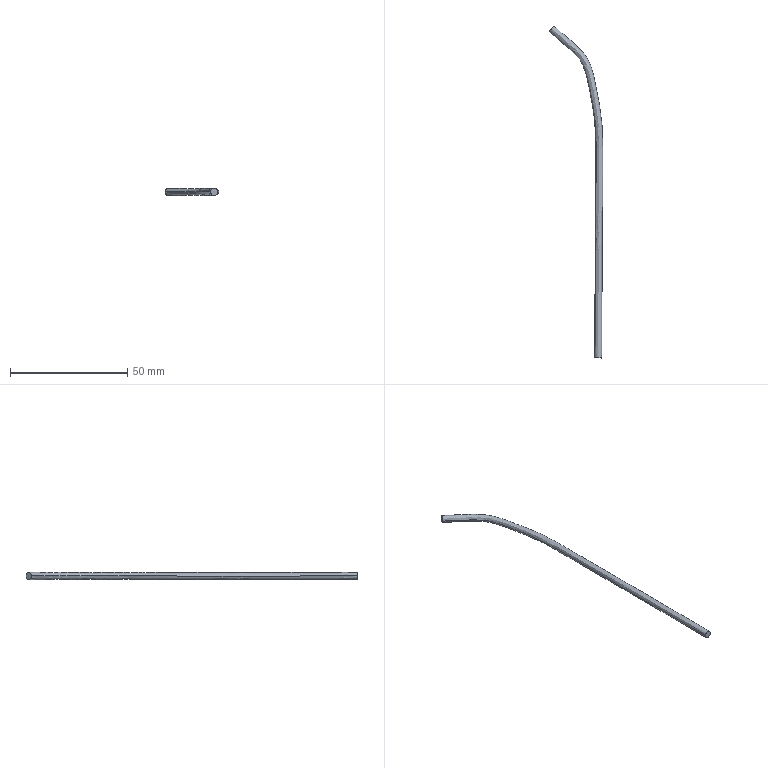Part | NX | features BREP 1 | 1 solid | 4 faces | box 22.885 x 141.616 x 3 mm | volume 1044 mm3 | plane 2 | spline 2
STEP:
#1=CARTESIAN_POINT('',(-420.73,-36.322,217.465));
#2=VERTEX_POINT('',#1);
#3=CARTESIAN_POINT('',(-417.73,-36.348,217.465));
#4=VERTEX_POINT('',#3);
#5=CARTESIAN_POINT('',(-420.73,-36.322,217.465));
#6=CARTESIAN_POINT('',(-420.73,-36.322,217.819));
#7=CARTESIAN_POINT('',(-420.462,-36.324,218.592));
#8=CARTESIAN_POINT('',(-419.23,-36.335,219.152));
#9=CARTESIAN_POINT('',(-417.998,-36.346,218.592));
#10=CARTESIAN_POINT('',(-417.73,-36.348,217.819));
#11=CARTESIAN_POINT('',(-417.73,-36.348,217.465));
#12=B_SPLINE_CURVE_WITH_KNOTS('',3,(#5,#6,#7,#8,#9,#10,#11),.UNSPECIFIED.,.F.,.F.,(4,1,1,1,4),(0.,0.25,0.5,0.75,1.),.UNSPECIFIED.);
#13=EDGE_CURVE('',#2,#4,#12,.T.);
#14=ORIENTED_EDGE('',*,*,#13,.F.);
#15=CARTESIAN_POINT('',(-417.73,-36.348,217.465));
#16=CARTESIAN_POINT('',(-417.73,-36.348,217.111));
#17=CARTESIAN_POINT('',(-417.998,-36.346,216.338));
#18=CARTESIAN_POINT('',(-419.23,-36.335,215.778));
#19=CARTESIAN_POINT('',(-420.462,-36.324,216.338));
#20=CARTESIAN_POINT('',(-420.73,-36.322,217.111));
#21=CARTESIAN_POINT('',(-420.73,-36.322,217.465));
#22=B_SPLINE_CURVE_WITH_KNOTS('',3,(#15,#16,#17,#18,#19,#20,#21),.UNSPECIFIED.,.F.,.F.,(4,1,1,1,4),(0.,0.25,0.5,0.75,1.),.UNSPECIFIED.);
#23=EDGE_CURVE('',#4,#2,#22,.T.);
#24=ORIENTED_EDGE('',*,*,#23,.F.);
#25=EDGE_LOOP('',(#14,#24));
#26=FACE_BOUND('',#25,.T.);
#27=CARTESIAN_POINT('',(-420.73,-36.322,217.465));
#28=DIRECTION('',(-0.00868,-1.,0.000000073));
#29=DIRECTION('',(1.,-0.00868,0.));
#30=AXIS2_PLACEMENT_3D('',#27,#28,#29);
#31=PLANE('',#30);
#32=ADVANCED_FACE('',(#26),#31,.T.);
#33=CARTESIAN_POINT('',(-440.089,102.958,217.465));
#34=VERTEX_POINT('',#33);
#35=CARTESIAN_POINT('',(-440.089,102.958,217.465));
#36=CARTESIAN_POINT('',(-437.76,101.027,217.465));
#37=CARTESIAN_POINT('',(-434.135,98.068,217.465));
#38=CARTESIAN_POINT('',(-429.923,94.157,217.465));
#39=CARTESIAN_POINT('',(-427.314,91.442,217.465));
#40=CARTESIAN_POINT('',(-425.94,89.22,217.465));
#41=CARTESIAN_POINT('',(-424.875,86.525,217.465));
#42=CARTESIAN_POINT('',(-423.928,83.021,217.465));
#43=CARTESIAN_POINT('',(-422.954,78.578,217.465));
#44=CARTESIAN_POINT('',(-422.135,74.275,217.465));
#45=CARTESIAN_POINT('',(-421.511,70.592,217.465));
#46=CARTESIAN_POINT('',(-421.057,67.594,217.465));
#47=CARTESIAN_POINT('',(-420.63,64.437,217.465));
#48=CARTESIAN_POINT('',(-420.318,60.773,217.465));
#49=CARTESIAN_POINT('',(-420.173,54.748,217.465));
#50=CARTESIAN_POINT('',(-420.218,48.728,217.465));
#51=CARTESIAN_POINT('',(-420.284,42.013,217.465));
#52=CARTESIAN_POINT('',(-420.325,37.072,217.465));
#53=CARTESIAN_POINT('',(-420.352,32.484,217.465));
#54=CARTESIAN_POINT('',(-420.373,26.403,217.465));
#55=CARTESIAN_POINT('',(-420.381,19.13,217.465));
#56=CARTESIAN_POINT('',(-420.4,10.592,217.465));
#57=CARTESIAN_POINT('',(-420.456,1.527,217.465));
#58=CARTESIAN_POINT('',(-420.55,-7.686,217.465));
#59=CARTESIAN_POINT('',(-420.645,-17.411,217.465));
#60=CARTESIAN_POINT('',(-420.693,-27.14,217.465));
#61=CARTESIAN_POINT('',(-420.704,-33.28,217.465));
#62=CARTESIAN_POINT('',(-420.73,-36.322,217.465));
#63=B_SPLINE_CURVE_WITH_KNOTS('',3,(#35,#36,#37,#38,#39,#40,#41,#42,#43,#44,#45,#46,#47,#48,#49,#50,#51,#52,#53,#54,#55,#56,#57,#58,#59,#60,#61,#62),.UNSPECIFIED.,.F.,.F.,(4,1,1,1,1,1,1,1,1,1,1,1,1,1,1,1,1,1,1,1,1,1,1,1,1,4),(0.,0.0625,0.09375,0.125,0.1406,0.1562,0.1875,0.2188,0.25,0.2812,0.2969,0.3125,0.3438,0.375,0.4375,0.4688,0.5,0.5312,0.5625,0.625,0.6875,0.75,0.8125,0.875,0.9375,1.),.UNSPECIFIED.);
#64=EDGE_CURVE('',#34,#2,#63,.T.);
#65=ORIENTED_EDGE('',*,*,#64,.T.);
#66=ORIENTED_EDGE('',*,*,#13,.T.);
#67=CARTESIAN_POINT('',(-438.175,105.268,217.465));
#68=VERTEX_POINT('',#67);
#69=CARTESIAN_POINT('',(-417.73,-36.348,217.465));
#70=CARTESIAN_POINT('',(-417.704,-33.291,217.465));
#71=CARTESIAN_POINT('',(-417.693,-27.147,217.465));
#72=CARTESIAN_POINT('',(-417.646,-17.435,217.465));
#73=CARTESIAN_POINT('',(-417.55,-7.719,217.465));
#74=CARTESIAN_POINT('',(-417.456,1.501,217.465));
#75=CARTESIAN_POINT('',(-417.4,10.58,217.465));
#76=CARTESIAN_POINT('',(-417.381,19.128,217.465));
#77=CARTESIAN_POINT('',(-417.373,26.397,217.465));
#78=CARTESIAN_POINT('',(-417.352,32.47,217.465));
#79=CARTESIAN_POINT('',(-417.325,37.051,217.465));
#80=CARTESIAN_POINT('',(-417.284,41.985,217.465));
#81=CARTESIAN_POINT('',(-417.218,48.699,217.465));
#82=CARTESIAN_POINT('',(-417.174,54.752,217.465));
#83=CARTESIAN_POINT('',(-417.318,60.899,217.465));
#84=CARTESIAN_POINT('',(-417.649,64.794,217.465));
#85=CARTESIAN_POINT('',(-418.088,68.024,217.465));
#86=CARTESIAN_POINT('',(-418.549,71.072,217.465));
#87=CARTESIAN_POINT('',(-419.182,74.805,217.465));
#88=CARTESIAN_POINT('',(-420.015,79.176,217.465));
#89=CARTESIAN_POINT('',(-420.837,82.95,217.465));
#90=CARTESIAN_POINT('',(-421.617,85.946,217.465));
#91=CARTESIAN_POINT('',(-422.303,88.174,217.465));
#92=CARTESIAN_POINT('',(-423.199,90.482,217.465));
#93=CARTESIAN_POINT('',(-424.583,92.742,217.465));
#94=CARTESIAN_POINT('',(-426.192,94.574,217.465));
#95=CARTESIAN_POINT('',(-428.351,96.806,217.465));
#96=CARTESIAN_POINT('',(-431.102,99.349,217.465));
#97=CARTESIAN_POINT('',(-434.673,102.351,217.465));
#98=CARTESIAN_POINT('',(-436.992,104.287,217.465));
#99=CARTESIAN_POINT('',(-438.175,105.268,217.465));
#100=B_SPLINE_CURVE_WITH_KNOTS('',3,(#69,#70,#71,#72,#73,#74,#75,#76,#77,#78,#79,#80,#81,#82,#83,#84,#85,#86,#87,#88,#89,#90,#91,#92,#93,#94,#95,#96,#97,#98,#99),.UNSPECIFIED.,.F.,.F.,(4,1,1,1,1,1,1,1,1,1,1,1,1,1,1,1,1,1,1,1,1,1,1,1,1,1,1,1,4),(0.,0.0625,0.125,0.1875,0.25,0.3125,0.375,0.4375,0.4688,0.5,0.5312,0.5625,0.625,0.6562,0.6875,0.7031,0.7188,0.75,0.7812,0.8125,0.8281,0.8438,0.8594,0.875,0.8906,0.9062,0.9375,0.9688,1.),.UNSPECIFIED.);
#101=EDGE_CURVE('',#4,#68,#100,.T.);
#102=ORIENTED_EDGE('',*,*,#101,.T.);
#103=CARTESIAN_POINT('',(-440.089,102.958,217.465));
#104=CARTESIAN_POINT('',(-440.089,102.958,217.819));
#105=CARTESIAN_POINT('',(-439.918,103.165,218.592));
#106=CARTESIAN_POINT('',(-439.132,104.113,219.152));
#107=CARTESIAN_POINT('',(-438.346,105.061,218.592));
#108=CARTESIAN_POINT('',(-438.175,105.268,217.819));
#109=CARTESIAN_POINT('',(-438.175,105.268,217.465));
#110=B_SPLINE_CURVE_WITH_KNOTS('',3,(#103,#104,#105,#106,#107,#108,#109),.UNSPECIFIED.,.F.,.F.,(4,1,1,1,4),(0.,0.25,0.5,0.75,1.),.UNSPECIFIED.);
#111=EDGE_CURVE('',#34,#68,#110,.T.);
#112=ORIENTED_EDGE('',*,*,#111,.F.);
#113=EDGE_LOOP('',(#65,#66,#102,#112));
#114=FACE_BOUND('',#113,.T.);
#115=CARTESIAN_POINT('',(-417.73,-36.348,217.465));
#116=CARTESIAN_POINT('',(-417.73,-36.348,217.819));
#117=CARTESIAN_POINT('',(-417.998,-36.346,218.592));
#118=CARTESIAN_POINT('',(-419.23,-36.335,219.152));
#119=CARTESIAN_POINT('',(-420.462,-36.324,218.592));
#120=CARTESIAN_POINT('',(-420.73,-36.322,217.819));
#121=CARTESIAN_POINT('',(-420.73,-36.322,217.465));
#122=CARTESIAN_POINT('',(-417.704,-33.289,217.465));
#123=CARTESIAN_POINT('',(-417.704,-33.289,217.819));
#124=CARTESIAN_POINT('',(-417.972,-33.288,218.592));
#125=CARTESIAN_POINT('',(-419.204,-33.284,219.152));
#126=CARTESIAN_POINT('',(-420.435,-33.279,218.592));
#127=CARTESIAN_POINT('',(-420.704,-33.278,217.819));
#128=CARTESIAN_POINT('',(-420.704,-33.278,217.465));
#129=CARTESIAN_POINT('',(-417.693,-27.141,217.465));
#130=CARTESIAN_POINT('',(-417.693,-27.141,217.819));
#131=CARTESIAN_POINT('',(-417.961,-27.141,218.592));
#132=CARTESIAN_POINT('',(-419.193,-27.138,219.152));
#133=CARTESIAN_POINT('',(-420.425,-27.135,218.592));
#134=CARTESIAN_POINT('',(-420.693,-27.134,217.819));
#135=CARTESIAN_POINT('',(-420.693,-27.134,217.465));
#136=CARTESIAN_POINT('',(-417.646,-17.423,217.465));
#137=CARTESIAN_POINT('',(-417.646,-17.423,217.819));
#138=CARTESIAN_POINT('',(-417.914,-17.42,218.592));
#139=CARTESIAN_POINT('',(-419.145,-17.411,219.152));
#140=CARTESIAN_POINT('',(-420.377,-17.401,218.592));
#141=CARTESIAN_POINT('',(-420.645,-17.399,217.819));
#142=CARTESIAN_POINT('',(-420.645,-17.399,217.465));
#143=CARTESIAN_POINT('',(-417.55,-7.7,217.465));
#144=CARTESIAN_POINT('',(-417.55,-7.7,217.819));
#145=CARTESIAN_POINT('',(-417.818,-7.697,218.592));
#146=CARTESIAN_POINT('',(-419.05,-7.684,219.152));
#147=CARTESIAN_POINT('',(-420.282,-7.67,218.592));
#148=CARTESIAN_POINT('',(-420.55,-7.668,217.819));
#149=CARTESIAN_POINT('',(-420.55,-7.668,217.465));
#150=CARTESIAN_POINT('',(-417.46,1.186,217.465));
#151=CARTESIAN_POINT('',(-417.46,1.186,217.819));
#152=CARTESIAN_POINT('',(-417.728,1.188,218.592));
#153=CARTESIAN_POINT('',(-418.96,1.199,219.152));
#154=CARTESIAN_POINT('',(-420.191,1.209,218.592));
#155=CARTESIAN_POINT('',(-420.46,1.212,217.819));
#156=CARTESIAN_POINT('',(-420.46,1.212,217.465));
#157=CARTESIAN_POINT('',(-417.405,9.624,217.465));
#158=CARTESIAN_POINT('',(-417.405,9.624,217.819));
#159=CARTESIAN_POINT('',(-417.673,9.625,218.592));
#160=CARTESIAN_POINT('',(-418.905,9.631,219.152));
#161=CARTESIAN_POINT('',(-420.137,9.636,218.592));
#162=CARTESIAN_POINT('',(-420.405,9.637,217.819));
#163=CARTESIAN_POINT('',(-420.405,9.637,217.465));
#164=CARTESIAN_POINT('',(-417.384,17.302,217.465));
#165=CARTESIAN_POINT('',(-417.384,17.302,217.819));
#166=CARTESIAN_POINT('',(-417.652,17.302,218.592));
#167=CARTESIAN_POINT('',(-418.884,17.304,219.152));
#168=CARTESIAN_POINT('',(-420.115,17.305,218.592));
#169=CARTESIAN_POINT('',(-420.384,17.306,217.819));
#170=CARTESIAN_POINT('',(-420.384,17.306,217.465));
#171=CARTESIAN_POINT('',(-417.375,24.98,217.465));
#172=CARTESIAN_POINT('',(-417.375,24.98,217.819));
#173=CARTESIAN_POINT('',(-417.643,24.981,218.592));
#174=CARTESIAN_POINT('',(-418.875,24.982,219.152));
#175=CARTESIAN_POINT('',(-420.107,24.984,218.592));
#176=CARTESIAN_POINT('',(-420.375,24.984,217.819));
#177=CARTESIAN_POINT('',(-420.375,24.984,217.465));
#178=CARTESIAN_POINT('',(-417.356,31.92,217.465));
#179=CARTESIAN_POINT('',(-417.356,31.92,217.819));
#180=CARTESIAN_POINT('',(-417.625,31.921,218.592));
#181=CARTESIAN_POINT('',(-418.856,31.926,219.152));
#182=CARTESIAN_POINT('',(-420.088,31.931,218.592));
#183=CARTESIAN_POINT('',(-420.356,31.932,217.819));
#184=CARTESIAN_POINT('',(-420.356,31.932,217.465));
#185=CARTESIAN_POINT('',(-417.32,37.816,217.465));
#186=CARTESIAN_POINT('',(-417.32,37.816,217.819));
#187=CARTESIAN_POINT('',(-417.588,37.818,218.592));
#188=CARTESIAN_POINT('',(-418.82,37.827,219.152));
#189=CARTESIAN_POINT('',(-420.052,37.837,218.592));
#190=CARTESIAN_POINT('',(-420.32,37.839,217.819));
#191=CARTESIAN_POINT('',(-420.32,37.839,217.465));
#192=CARTESIAN_POINT('',(-417.275,42.946,217.465));
#193=CARTESIAN_POINT('',(-417.275,42.946,217.819));
#194=CARTESIAN_POINT('',(-417.543,42.949,218.592));
#195=CARTESIAN_POINT('',(-418.775,42.961,219.152));
#196=CARTESIAN_POINT('',(-420.006,42.973,218.592));
#197=CARTESIAN_POINT('',(-420.275,42.975,217.819));
#198=CARTESIAN_POINT('',(-420.275,42.975,217.465));
#199=CARTESIAN_POINT('',(-417.224,48.08,217.465));
#200=CARTESIAN_POINT('',(-417.224,48.08,217.819));
#201=CARTESIAN_POINT('',(-417.492,48.083,218.592));
#202=CARTESIAN_POINT('',(-418.724,48.094,219.152));
#203=CARTESIAN_POINT('',(-419.956,48.105,218.592));
#204=CARTESIAN_POINT('',(-420.224,48.107,217.819));
#205=CARTESIAN_POINT('',(-420.224,48.107,217.465));
#206=CARTESIAN_POINT('',(-417.198,52.103,217.465));
#207=CARTESIAN_POINT('',(-417.198,52.103,217.819));
#208=CARTESIAN_POINT('',(-417.467,52.104,218.592));
#209=CARTESIAN_POINT('',(-418.698,52.108,219.152));
#210=CARTESIAN_POINT('',(-419.93,52.112,218.592));
#211=CARTESIAN_POINT('',(-420.198,52.113,217.819));
#212=CARTESIAN_POINT('',(-420.198,52.113,217.465));
#213=CARTESIAN_POINT('',(-417.21,55.372,217.465));
#214=CARTESIAN_POINT('',(-417.21,55.372,217.819));
#215=CARTESIAN_POINT('',(-417.478,55.369,218.592));
#216=CARTESIAN_POINT('',(-418.71,55.359,219.152));
#217=CARTESIAN_POINT('',(-419.942,55.348,218.592));
#218=CARTESIAN_POINT('',(-420.21,55.346,217.819));
#219=CARTESIAN_POINT('',(-420.21,55.346,217.465));
#220=CARTESIAN_POINT('',(-417.262,58.768,217.465));
#221=CARTESIAN_POINT('',(-417.262,58.768,217.819));
#222=CARTESIAN_POINT('',(-417.531,58.76,218.592));
#223=CARTESIAN_POINT('',(-418.762,58.726,219.152));
#224=CARTESIAN_POINT('',(-419.993,58.692,218.592));
#225=CARTESIAN_POINT('',(-420.261,58.684,217.819));
#226=CARTESIAN_POINT('',(-420.261,58.684,217.465));
#227=CARTESIAN_POINT('',(-417.39,61.891,217.465));
#228=CARTESIAN_POINT('',(-417.39,61.891,217.819));
#229=CARTESIAN_POINT('',(-417.658,61.875,218.592));
#230=CARTESIAN_POINT('',(-418.888,61.801,219.152));
#231=CARTESIAN_POINT('',(-420.118,61.727,218.592));
#232=CARTESIAN_POINT('',(-420.386,61.711,217.819));
#233=CARTESIAN_POINT('',(-420.386,61.711,217.465));
#234=CARTESIAN_POINT('',(-417.669,64.766,217.465));
#235=CARTESIAN_POINT('',(-417.669,64.766,217.819));
#236=CARTESIAN_POINT('',(-417.935,64.736,218.592));
#237=CARTESIAN_POINT('',(-419.16,64.597,219.152));
#238=CARTESIAN_POINT('',(-420.384,64.458,218.592));
#239=CARTESIAN_POINT('',(-420.65,64.427,217.819));
#240=CARTESIAN_POINT('',(-420.65,64.427,217.465));
#241=CARTESIAN_POINT('',(-417.883,66.521,217.465));
#242=CARTESIAN_POINT('',(-417.883,66.521,217.819));
#243=CARTESIAN_POINT('',(-418.149,66.485,218.592));
#244=CARTESIAN_POINT('',(-419.37,66.321,219.152));
#245=CARTESIAN_POINT('',(-420.591,66.157,218.592));
#246=CARTESIAN_POINT('',(-420.857,66.122,217.819));
#247=CARTESIAN_POINT('',(-420.857,66.122,217.465));
#248=CARTESIAN_POINT('',(-418.124,68.258,217.465));
#249=CARTESIAN_POINT('',(-418.124,68.258,217.819));
#250=CARTESIAN_POINT('',(-418.39,68.219,218.592));
#251=CARTESIAN_POINT('',(-419.609,68.042,219.152));
#252=CARTESIAN_POINT('',(-420.828,67.864,218.592));
#253=CARTESIAN_POINT('',(-421.093,67.825,217.819));
#254=CARTESIAN_POINT('',(-421.093,67.825,217.465));
#255=CARTESIAN_POINT('',(-418.618,71.527,217.465));
#256=CARTESIAN_POINT('',(-418.618,71.527,217.819));
#257=CARTESIAN_POINT('',(-418.882,71.484,218.592));
#258=CARTESIAN_POINT('',(-420.098,71.283,219.152));
#259=CARTESIAN_POINT('',(-421.313,71.083,218.592));
#260=CARTESIAN_POINT('',(-421.578,71.039,217.819));
#261=CARTESIAN_POINT('',(-421.578,71.039,217.465));
#262=CARTESIAN_POINT('',(-419.253,75.208,217.465));
#263=CARTESIAN_POINT('',(-419.253,75.208,217.819));
#264=CARTESIAN_POINT('',(-419.517,75.16,218.592));
#265=CARTESIAN_POINT('',(-420.729,74.94,219.152));
#266=CARTESIAN_POINT('',(-421.941,74.721,218.592));
#267=CARTESIAN_POINT('',(-422.205,74.673,217.819));
#268=CARTESIAN_POINT('',(-422.205,74.673,217.465));
#269=CARTESIAN_POINT('',(-420.057,79.337,217.465));
#270=CARTESIAN_POINT('',(-420.057,79.337,217.819));
#271=CARTESIAN_POINT('',(-420.32,79.284,218.592));
#272=CARTESIAN_POINT('',(-421.527,79.037,219.152));
#273=CARTESIAN_POINT('',(-422.734,78.791,218.592));
#274=CARTESIAN_POINT('',(-422.997,78.737,217.819));
#275=CARTESIAN_POINT('',(-422.997,78.737,217.465));
#276=CARTESIAN_POINT('',(-420.761,82.605,217.465));
#277=CARTESIAN_POINT('',(-420.761,82.605,217.819));
#278=CARTESIAN_POINT('',(-421.023,82.545,218.592));
#279=CARTESIAN_POINT('',(-422.224,82.269,219.152));
#280=CARTESIAN_POINT('',(-423.424,81.993,218.592));
#281=CARTESIAN_POINT('',(-423.686,81.932,217.819));
#282=CARTESIAN_POINT('',(-423.686,81.932,217.465));
#283=CARTESIAN_POINT('',(-421.595,85.934,217.465));
#284=CARTESIAN_POINT('',(-421.595,85.934,217.819));
#285=CARTESIAN_POINT('',(-421.854,85.863,218.592));
#286=CARTESIAN_POINT('',(-423.042,85.537,219.152));
#287=CARTESIAN_POINT('',(-424.23,85.21,218.592));
#288=CARTESIAN_POINT('',(-424.488,85.139,217.819));
#289=CARTESIAN_POINT('',(-424.488,85.139,217.465));
#290=CARTESIAN_POINT('',(-422.417,88.543,217.465));
#291=CARTESIAN_POINT('',(-422.417,88.543,217.819));
#292=CARTESIAN_POINT('',(-422.67,88.453,218.592));
#293=CARTESIAN_POINT('',(-423.832,88.038,219.152));
#294=CARTESIAN_POINT('',(-424.994,87.624,218.592));
#295=CARTESIAN_POINT('',(-425.248,87.534,217.819));
#296=CARTESIAN_POINT('',(-425.248,87.534,217.465));
#297=CARTESIAN_POINT('',(-423.245,90.439,217.465));
#298=CARTESIAN_POINT('',(-423.245,90.439,217.819));
#299=CARTESIAN_POINT('',(-423.488,90.324,218.592));
#300=CARTESIAN_POINT('',(-424.602,89.795,219.152));
#301=CARTESIAN_POINT('',(-425.717,89.266,218.592));
#302=CARTESIAN_POINT('',(-425.959,89.151,217.819));
#303=CARTESIAN_POINT('',(-425.959,89.151,217.465));
#304=CARTESIAN_POINT('',(-423.977,91.809,217.465));
#305=CARTESIAN_POINT('',(-423.977,91.809,217.819));
#306=CARTESIAN_POINT('',(-424.204,91.664,218.592));
#307=CARTESIAN_POINT('',(-425.245,90.999,219.152));
#308=CARTESIAN_POINT('',(-426.287,90.334,218.592));
#309=CARTESIAN_POINT('',(-426.514,90.189,217.819));
#310=CARTESIAN_POINT('',(-426.514,90.189,217.465));
#311=CARTESIAN_POINT('',(-425.026,93.246,217.465));
#312=CARTESIAN_POINT('',(-425.026,93.246,217.819));
#313=CARTESIAN_POINT('',(-425.234,93.074,218.592));
#314=CARTESIAN_POINT('',(-426.185,92.288,219.152));
#315=CARTESIAN_POINT('',(-427.136,91.502,218.592));
#316=CARTESIAN_POINT('',(-427.343,91.33,217.819));
#317=CARTESIAN_POINT('',(-427.343,91.33,217.465));
#318=CARTESIAN_POINT('',(-426.79,95.236,217.465));
#319=CARTESIAN_POINT('',(-426.79,95.236,217.819));
#320=CARTESIAN_POINT('',(-426.983,95.049,218.592));
#321=CARTESIAN_POINT('',(-427.866,94.19,219.152));
#322=CARTESIAN_POINT('',(-428.75,93.331,218.592));
#323=CARTESIAN_POINT('',(-428.942,93.144,217.819));
#324=CARTESIAN_POINT('',(-428.942,93.144,217.465));
#325=CARTESIAN_POINT('',(-428.587,97.008,217.465));
#326=CARTESIAN_POINT('',(-428.587,97.008,217.819));
#327=CARTESIAN_POINT('',(-428.773,96.814,218.592));
#328=CARTESIAN_POINT('',(-429.626,95.926,219.152));
#329=CARTESIAN_POINT('',(-430.479,95.038,218.592));
#330=CARTESIAN_POINT('',(-430.665,94.845,217.819));
#331=CARTESIAN_POINT('',(-430.665,94.845,217.465));
#332=CARTESIAN_POINT('',(-430.429,98.709,217.465));
#333=CARTESIAN_POINT('',(-430.429,98.709,217.819));
#334=CARTESIAN_POINT('',(-430.609,98.51,218.592));
#335=CARTESIAN_POINT('',(-431.434,97.595,219.152));
#336=CARTESIAN_POINT('',(-432.259,96.68,218.592));
#337=CARTESIAN_POINT('',(-432.438,96.481,217.819));
#338=CARTESIAN_POINT('',(-432.438,96.481,217.465));
#339=CARTESIAN_POINT('',(-432.432,100.478,217.465));
#340=CARTESIAN_POINT('',(-432.432,100.478,217.819));
#341=CARTESIAN_POINT('',(-432.606,100.273,218.592));
#342=CARTESIAN_POINT('',(-433.405,99.336,219.152));
#343=CARTESIAN_POINT('',(-434.204,98.398,218.592));
#344=CARTESIAN_POINT('',(-434.378,98.194,217.819));
#345=CARTESIAN_POINT('',(-434.378,98.194,217.465));
#346=CARTESIAN_POINT('',(-435.037,102.65,217.465));
#347=CARTESIAN_POINT('',(-435.037,102.65,217.819));
#348=CARTESIAN_POINT('',(-435.208,102.443,218.592));
#349=CARTESIAN_POINT('',(-435.991,101.492,219.152));
#350=CARTESIAN_POINT('',(-436.773,100.541,218.592));
#351=CARTESIAN_POINT('',(-436.944,100.334,217.819));
#352=CARTESIAN_POINT('',(-436.944,100.334,217.465));
#353=CARTESIAN_POINT('',(-437.116,104.391,217.465));
#354=CARTESIAN_POINT('',(-437.116,104.391,217.819));
#355=CARTESIAN_POINT('',(-437.289,104.185,218.592));
#356=CARTESIAN_POINT('',(-438.082,103.243,219.152));
#357=CARTESIAN_POINT('',(-438.875,102.3,218.592));
#358=CARTESIAN_POINT('',(-439.047,102.095,217.819));
#359=CARTESIAN_POINT('',(-439.047,102.095,217.465));
#360=CARTESIAN_POINT('',(-438.175,105.268,217.465));
#361=CARTESIAN_POINT('',(-438.175,105.268,217.819));
#362=CARTESIAN_POINT('',(-438.346,105.061,218.592));
#363=CARTESIAN_POINT('',(-439.132,104.113,219.152));
#364=CARTESIAN_POINT('',(-439.918,103.165,218.592));
#365=CARTESIAN_POINT('',(-440.089,102.958,217.819));
#366=CARTESIAN_POINT('',(-440.089,102.958,217.465));
#367=B_SPLINE_SURFACE_WITH_KNOTS('',3,3,((#115,#116,#117,#118,#119,#120,#121),(#122,#123,#124,#125,#126,#127,#128),(#129,#130,#131,#132,#133,#134,#135),(#136,#137,#138,#139,#140,#141,#142),(#143,#144,#145,#146,#147,#148,#149),(#150,#151,#152,#153,#154,#155,#156),(#157,#158,#159,#160,#161,#162,#163),(#164,#165,#166,#167,#168,#169,#170),(#171,#172,#173,#174,#175,#176,#177),(#178,#179,#180,#181,#182,#183,#184),(#185,#186,#187,#188,#189,#190,#191),(#192,#193,#194,#195,#196,#197,#198),(#199,#200,#201,#202,#203,#204,#205),(#206,#207,#208,#209,#210,#211,#212),(#213,#214,#215,#216,#217,#218,#219),(#220,#221,#222,#223,#224,#225,#226),(#227,#228,#229,#230,#231,#232,#233),(#234,#235,#236,#237,#238,#239,#240),(#241,#242,#243,#244,#245,#246,#247),(#248,#249,#250,#251,#252,#253,#254),(#255,#256,#257,#258,#259,#260,#261),(#262,#263,#264,#265,#266,#267,#268),(#269,#270,#271,#272,#273,#274,#275),(#276,#277,#278,#279,#280,#281,#282),(#283,#284,#285,#286,#287,#288,#289),(#290,#291,#292,#293,#294,#295,#296),(#297,#298,#299,#300,#301,#302,#303),(#304,#305,#306,#307,#308,#309,#310),(#311,#312,#313,#314,#315,#316,#317),(#318,#319,#320,#321,#322,#323,#324),(#325,#326,#327,#328,#329,#330,#331),(#332,#333,#334,#335,#336,#337,#338),(#339,#340,#341,#342,#343,#344,#345),(#346,#347,#348,#349,#350,#351,#352),(#353,#354,#355,#356,#357,#358,#359),(#360,#361,#362,#363,#364,#365,#366)),.UNSPECIFIED.,.F.,.F.,.F.,(4,1,1,1,1,1,1,1,1,1,1,1,1,1,1,1,1,1,1,1,1,1,1,1,1,1,1,1,1,1,1,1,1,4),(4,1,1,1,4),(0.009816,0.07113,0.1324,0.1938,0.2551,0.3097,0.3643,0.4189,0.4735,0.505,0.5364,0.5679,0.5994,0.6164,0.6334,0.6673,0.6785,0.6896,0.7007,0.7119,0.7551,0.7768,0.7984,0.8216,0.8448,0.8521,0.8594,0.8719,0.8843,0.9098,0.9226,0.9354,0.9628,0.9902),(0.02179,0.261,0.5002,0.7394,0.9786),.UNSPECIFIED.);
#368=ADVANCED_FACE('',(#114),#367,.T.);
#369=ORIENTED_EDGE('',*,*,#101,.F.);
#370=ORIENTED_EDGE('',*,*,#23,.T.);
#371=ORIENTED_EDGE('',*,*,#64,.F.);
#372=CARTESIAN_POINT('',(-438.175,105.268,217.465));
#373=CARTESIAN_POINT('',(-438.175,105.268,217.111));
#374=CARTESIAN_POINT('',(-438.346,105.061,216.338));
#375=CARTESIAN_POINT('',(-439.132,104.113,215.778));
#376=CARTESIAN_POINT('',(-439.918,103.165,216.338));
#377=CARTESIAN_POINT('',(-440.089,102.958,217.111));
#378=CARTESIAN_POINT('',(-440.089,102.958,217.465));
#379=B_SPLINE_CURVE_WITH_KNOTS('',3,(#372,#373,#374,#375,#376,#377,#378),.UNSPECIFIED.,.F.,.F.,(4,1,1,1,4),(0.,0.25,0.5,0.75,1.),.UNSPECIFIED.);
#380=EDGE_CURVE('',#68,#34,#379,.T.);
#381=ORIENTED_EDGE('',*,*,#380,.F.);
#382=EDGE_LOOP('',(#369,#370,#371,#381));
#383=FACE_BOUND('',#382,.T.);
#384=CARTESIAN_POINT('',(-420.73,-36.322,217.465));
#385=CARTESIAN_POINT('',(-420.73,-36.322,217.111));
#386=CARTESIAN_POINT('',(-420.462,-36.324,216.338));
#387=CARTESIAN_POINT('',(-419.23,-36.335,215.778));
#388=CARTESIAN_POINT('',(-417.998,-36.346,216.338));
#389=CARTESIAN_POINT('',(-417.73,-36.348,217.111));
#390=CARTESIAN_POINT('',(-417.73,-36.348,217.465));
#391=CARTESIAN_POINT('',(-420.704,-33.278,217.465));
#392=CARTESIAN_POINT('',(-420.704,-33.278,217.111));
#393=CARTESIAN_POINT('',(-420.435,-33.279,216.338));
#394=CARTESIAN_POINT('',(-419.204,-33.284,215.778));
#395=CARTESIAN_POINT('',(-417.972,-33.288,216.338));
#396=CARTESIAN_POINT('',(-417.704,-33.289,217.111));
#397=CARTESIAN_POINT('',(-417.704,-33.289,217.465));
#398=CARTESIAN_POINT('',(-420.693,-27.134,217.465));
#399=CARTESIAN_POINT('',(-420.693,-27.134,217.111));
#400=CARTESIAN_POINT('',(-420.425,-27.135,216.338));
#401=CARTESIAN_POINT('',(-419.193,-27.138,215.778));
#402=CARTESIAN_POINT('',(-417.961,-27.141,216.338));
#403=CARTESIAN_POINT('',(-417.693,-27.141,217.111));
#404=CARTESIAN_POINT('',(-417.693,-27.141,217.465));
#405=CARTESIAN_POINT('',(-420.645,-17.399,217.465));
#406=CARTESIAN_POINT('',(-420.645,-17.399,217.111));
#407=CARTESIAN_POINT('',(-420.377,-17.401,216.338));
#408=CARTESIAN_POINT('',(-419.145,-17.411,215.778));
#409=CARTESIAN_POINT('',(-417.914,-17.42,216.338));
#410=CARTESIAN_POINT('',(-417.646,-17.423,217.111));
#411=CARTESIAN_POINT('',(-417.646,-17.423,217.465));
#412=CARTESIAN_POINT('',(-420.55,-7.668,217.465));
#413=CARTESIAN_POINT('',(-420.55,-7.668,217.111));
#414=CARTESIAN_POINT('',(-420.282,-7.67,216.338));
#415=CARTESIAN_POINT('',(-419.05,-7.684,215.778));
#416=CARTESIAN_POINT('',(-417.818,-7.697,216.338));
#417=CARTESIAN_POINT('',(-417.55,-7.7,217.111));
#418=CARTESIAN_POINT('',(-417.55,-7.7,217.465));
#419=CARTESIAN_POINT('',(-420.46,1.212,217.465));
#420=CARTESIAN_POINT('',(-420.46,1.212,217.111));
#421=CARTESIAN_POINT('',(-420.191,1.209,216.338));
#422=CARTESIAN_POINT('',(-418.96,1.199,215.778));
#423=CARTESIAN_POINT('',(-417.728,1.188,216.338));
#424=CARTESIAN_POINT('',(-417.46,1.186,217.111));
#425=CARTESIAN_POINT('',(-417.46,1.186,217.465));
#426=CARTESIAN_POINT('',(-420.405,9.637,217.465));
#427=CARTESIAN_POINT('',(-420.405,9.637,217.111));
#428=CARTESIAN_POINT('',(-420.137,9.636,216.338));
#429=CARTESIAN_POINT('',(-418.905,9.631,215.778));
#430=CARTESIAN_POINT('',(-417.673,9.625,216.338));
#431=CARTESIAN_POINT('',(-417.405,9.624,217.111));
#432=CARTESIAN_POINT('',(-417.405,9.624,217.465));
#433=CARTESIAN_POINT('',(-420.384,17.306,217.465));
#434=CARTESIAN_POINT('',(-420.384,17.306,217.111));
#435=CARTESIAN_POINT('',(-420.115,17.305,216.338));
#436=CARTESIAN_POINT('',(-418.884,17.304,215.778));
#437=CARTESIAN_POINT('',(-417.652,17.302,216.338));
#438=CARTESIAN_POINT('',(-417.384,17.302,217.111));
#439=CARTESIAN_POINT('',(-417.384,17.302,217.465));
#440=CARTESIAN_POINT('',(-420.375,24.984,217.465));
#441=CARTESIAN_POINT('',(-420.375,24.984,217.111));
#442=CARTESIAN_POINT('',(-420.107,24.984,216.338));
#443=CARTESIAN_POINT('',(-418.875,24.982,215.778));
#444=CARTESIAN_POINT('',(-417.643,24.981,216.338));
#445=CARTESIAN_POINT('',(-417.375,24.98,217.111));
#446=CARTESIAN_POINT('',(-417.375,24.98,217.465));
#447=CARTESIAN_POINT('',(-420.356,31.932,217.465));
#448=CARTESIAN_POINT('',(-420.356,31.932,217.111));
#449=CARTESIAN_POINT('',(-420.088,31.931,216.338));
#450=CARTESIAN_POINT('',(-418.856,31.926,215.778));
#451=CARTESIAN_POINT('',(-417.625,31.921,216.338));
#452=CARTESIAN_POINT('',(-417.356,31.92,217.111));
#453=CARTESIAN_POINT('',(-417.356,31.92,217.465));
#454=CARTESIAN_POINT('',(-420.32,37.839,217.465));
#455=CARTESIAN_POINT('',(-420.32,37.839,217.111));
#456=CARTESIAN_POINT('',(-420.052,37.837,216.338));
#457=CARTESIAN_POINT('',(-418.82,37.827,215.778));
#458=CARTESIAN_POINT('',(-417.588,37.818,216.338));
#459=CARTESIAN_POINT('',(-417.32,37.816,217.111));
#460=CARTESIAN_POINT('',(-417.32,37.816,217.465));
#461=CARTESIAN_POINT('',(-420.275,42.975,217.465));
#462=CARTESIAN_POINT('',(-420.275,42.975,217.111));
#463=CARTESIAN_POINT('',(-420.006,42.973,216.338));
#464=CARTESIAN_POINT('',(-418.775,42.961,215.778));
#465=CARTESIAN_POINT('',(-417.543,42.949,216.338));
#466=CARTESIAN_POINT('',(-417.275,42.946,217.111));
#467=CARTESIAN_POINT('',(-417.275,42.946,217.465));
#468=CARTESIAN_POINT('',(-420.224,48.107,217.465));
#469=CARTESIAN_POINT('',(-420.224,48.107,217.111));
#470=CARTESIAN_POINT('',(-419.956,48.105,216.338));
#471=CARTESIAN_POINT('',(-418.724,48.094,215.778));
#472=CARTESIAN_POINT('',(-417.492,48.083,216.338));
#473=CARTESIAN_POINT('',(-417.224,48.08,217.111));
#474=CARTESIAN_POINT('',(-417.224,48.08,217.465));
#475=CARTESIAN_POINT('',(-420.198,52.113,217.465));
#476=CARTESIAN_POINT('',(-420.198,52.113,217.111));
#477=CARTESIAN_POINT('',(-419.93,52.112,216.338));
#478=CARTESIAN_POINT('',(-418.698,52.108,215.778));
#479=CARTESIAN_POINT('',(-417.466,52.104,216.338));
#480=CARTESIAN_POINT('',(-417.198,52.103,217.111));
#481=CARTESIAN_POINT('',(-417.198,52.103,217.465));
#482=CARTESIAN_POINT('',(-420.21,55.346,217.465));
#483=CARTESIAN_POINT('',(-420.21,55.346,217.111));
#484=CARTESIAN_POINT('',(-419.942,55.348,216.338));
#485=CARTESIAN_POINT('',(-418.71,55.359,215.778));
#486=CARTESIAN_POINT('',(-417.478,55.369,216.338));
#487=CARTESIAN_POINT('',(-417.21,55.372,217.111));
#488=CARTESIAN_POINT('',(-417.21,55.372,217.465));
#489=CARTESIAN_POINT('',(-420.248,57.85,217.465));
#490=CARTESIAN_POINT('',(-420.248,57.85,217.111));
#491=CARTESIAN_POINT('',(-419.98,57.856,216.338));
#492=CARTESIAN_POINT('',(-418.748,57.884,215.778));
#493=CARTESIAN_POINT('',(-417.517,57.913,216.338));
#494=CARTESIAN_POINT('',(-417.249,57.919,217.111));
#495=CARTESIAN_POINT('',(-417.249,57.919,217.465));
#496=CARTESIAN_POINT('',(-420.331,60.34,217.465));
#497=CARTESIAN_POINT('',(-420.331,60.34,217.111));
#498=CARTESIAN_POINT('',(-420.063,60.352,216.338));
#499=CARTESIAN_POINT('',(-418.833,60.408,215.778));
#500=CARTESIAN_POINT('',(-417.602,60.464,216.338));
#501=CARTESIAN_POINT('',(-417.334,60.476,217.111));
#502=CARTESIAN_POINT('',(-417.334,60.476,217.465));
#503=CARTESIAN_POINT('',(-420.466,62.531,217.465));
#504=CARTESIAN_POINT('',(-420.466,62.531,217.111));
#505=CARTESIAN_POINT('',(-420.198,62.551,216.338));
#506=CARTESIAN_POINT('',(-418.97,62.645,215.778));
#507=CARTESIAN_POINT('',(-417.741,62.739,216.338));
#508=CARTESIAN_POINT('',(-417.474,62.759,217.111));
#509=CARTESIAN_POINT('',(-417.474,62.759,217.465));
#510=CARTESIAN_POINT('',(-420.65,64.427,217.465));
#511=CARTESIAN_POINT('',(-420.65,64.427,217.111));
#512=CARTESIAN_POINT('',(-420.384,64.458,216.338));
#513=CARTESIAN_POINT('',(-419.16,64.597,215.778));
#514=CARTESIAN_POINT('',(-417.936,64.736,216.338));
#515=CARTESIAN_POINT('',(-417.669,64.766,217.111));
#516=CARTESIAN_POINT('',(-417.669,64.766,217.465));
#517=CARTESIAN_POINT('',(-420.857,66.122,217.465));
#518=CARTESIAN_POINT('',(-420.857,66.122,217.111));
#519=CARTESIAN_POINT('',(-420.591,66.157,216.338));
#520=CARTESIAN_POINT('',(-419.37,66.321,215.778));
#521=CARTESIAN_POINT('',(-418.149,66.485,216.338));
#522=CARTESIAN_POINT('',(-417.883,66.521,217.111));
#523=CARTESIAN_POINT('',(-417.883,66.521,217.465));
#524=CARTESIAN_POINT('',(-421.093,67.825,217.465));
#525=CARTESIAN_POINT('',(-421.093,67.825,217.111));
#526=CARTESIAN_POINT('',(-420.828,67.864,216.338));
#527=CARTESIAN_POINT('',(-419.609,68.042,215.778));
#528=CARTESIAN_POINT('',(-418.39,68.219,216.338));
#529=CARTESIAN_POINT('',(-418.124,68.258,217.111));
#530=CARTESIAN_POINT('',(-418.124,68.258,217.465));
#531=CARTESIAN_POINT('',(-421.578,71.039,217.465));
#532=CARTESIAN_POINT('',(-421.578,71.039,217.111));
#533=CARTESIAN_POINT('',(-421.313,71.083,216.338));
#534=CARTESIAN_POINT('',(-420.098,71.283,215.778));
#535=CARTESIAN_POINT('',(-418.882,71.484,216.338));
#536=CARTESIAN_POINT('',(-418.618,71.527,217.111));
#537=CARTESIAN_POINT('',(-418.618,71.527,217.465));
#538=CARTESIAN_POINT('',(-422.205,74.673,217.465));
#539=CARTESIAN_POINT('',(-422.205,74.673,217.111));
#540=CARTESIAN_POINT('',(-421.941,74.721,216.338));
#541=CARTESIAN_POINT('',(-420.729,74.94,215.778));
#542=CARTESIAN_POINT('',(-419.517,75.16,216.338));
#543=CARTESIAN_POINT('',(-419.253,75.208,217.111));
#544=CARTESIAN_POINT('',(-419.253,75.208,217.465));
#545=CARTESIAN_POINT('',(-422.997,78.737,217.465));
#546=CARTESIAN_POINT('',(-422.997,78.737,217.111));
#547=CARTESIAN_POINT('',(-422.734,78.791,216.338));
#548=CARTESIAN_POINT('',(-421.527,79.037,215.778));
#549=CARTESIAN_POINT('',(-420.32,79.284,216.338));
#550=CARTESIAN_POINT('',(-420.057,79.337,217.111));
#551=CARTESIAN_POINT('',(-420.057,79.337,217.465));
#552=CARTESIAN_POINT('',(-423.686,81.932,217.465));
#553=CARTESIAN_POINT('',(-423.686,81.932,217.111));
#554=CARTESIAN_POINT('',(-423.424,81.993,216.338));
#555=CARTESIAN_POINT('',(-422.224,82.269,215.778));
#556=CARTESIAN_POINT('',(-421.023,82.545,216.338));
#557=CARTESIAN_POINT('',(-420.761,82.605,217.111));
#558=CARTESIAN_POINT('',(-420.761,82.605,217.465));
#559=CARTESIAN_POINT('',(-424.488,85.139,217.465));
#560=CARTESIAN_POINT('',(-424.488,85.139,217.111));
#561=CARTESIAN_POINT('',(-424.23,85.21,216.338));
#562=CARTESIAN_POINT('',(-423.042,85.537,215.778));
#563=CARTESIAN_POINT('',(-421.854,85.863,216.338));
#564=CARTESIAN_POINT('',(-421.595,85.934,217.111));
#565=CARTESIAN_POINT('',(-421.595,85.934,217.465));
#566=CARTESIAN_POINT('',(-425.248,87.534,217.465));
#567=CARTESIAN_POINT('',(-425.248,87.534,217.111));
#568=CARTESIAN_POINT('',(-424.994,87.624,216.338));
#569=CARTESIAN_POINT('',(-423.832,88.038,215.778));
#570=CARTESIAN_POINT('',(-422.67,88.453,216.338));
#571=CARTESIAN_POINT('',(-422.417,88.543,217.111));
#572=CARTESIAN_POINT('',(-422.417,88.543,217.465));
#573=CARTESIAN_POINT('',(-425.959,89.151,217.465));
#574=CARTESIAN_POINT('',(-425.959,89.151,217.111));
#575=CARTESIAN_POINT('',(-425.717,89.266,216.338));
#576=CARTESIAN_POINT('',(-424.602,89.795,215.778));
#577=CARTESIAN_POINT('',(-423.488,90.324,216.338));
#578=CARTESIAN_POINT('',(-423.245,90.439,217.111));
#579=CARTESIAN_POINT('',(-423.245,90.439,217.465));
#580=CARTESIAN_POINT('',(-426.514,90.189,217.465));
#581=CARTESIAN_POINT('',(-426.514,90.189,217.111));
#582=CARTESIAN_POINT('',(-426.287,90.334,216.338));
#583=CARTESIAN_POINT('',(-425.245,90.999,215.778));
#584=CARTESIAN_POINT('',(-424.204,91.664,216.338));
#585=CARTESIAN_POINT('',(-423.977,91.809,217.111));
#586=CARTESIAN_POINT('',(-423.977,91.809,217.465));
#587=CARTESIAN_POINT('',(-427.343,91.33,217.465));
#588=CARTESIAN_POINT('',(-427.343,91.33,217.111));
#589=CARTESIAN_POINT('',(-427.136,91.502,216.338));
#590=CARTESIAN_POINT('',(-426.185,92.288,215.778));
#591=CARTESIAN_POINT('',(-425.234,93.074,216.338));
#592=CARTESIAN_POINT('',(-425.026,93.246,217.111));
#593=CARTESIAN_POINT('',(-425.026,93.246,217.465));
#594=CARTESIAN_POINT('',(-428.942,93.144,217.465));
#595=CARTESIAN_POINT('',(-428.942,93.144,217.111));
#596=CARTESIAN_POINT('',(-428.75,93.331,216.338));
#597=CARTESIAN_POINT('',(-427.866,94.19,215.778));
#598=CARTESIAN_POINT('',(-426.983,95.049,216.338));
#599=CARTESIAN_POINT('',(-426.79,95.236,217.111));
#600=CARTESIAN_POINT('',(-426.79,95.236,217.465));
#601=CARTESIAN_POINT('',(-430.665,94.845,217.465));
#602=CARTESIAN_POINT('',(-430.665,94.845,217.111));
#603=CARTESIAN_POINT('',(-430.479,95.038,216.338));
#604=CARTESIAN_POINT('',(-429.626,95.926,215.778));
#605=CARTESIAN_POINT('',(-428.773,96.814,216.338));
#606=CARTESIAN_POINT('',(-428.587,97.008,217.111));
#607=CARTESIAN_POINT('',(-428.587,97.008,217.465));
#608=CARTESIAN_POINT('',(-432.438,96.481,217.465));
#609=CARTESIAN_POINT('',(-432.438,96.481,217.111));
#610=CARTESIAN_POINT('',(-432.259,96.68,216.338));
#611=CARTESIAN_POINT('',(-431.434,97.595,215.778));
#612=CARTESIAN_POINT('',(-430.609,98.51,216.338));
#613=CARTESIAN_POINT('',(-430.429,98.709,217.111));
#614=CARTESIAN_POINT('',(-430.429,98.709,217.465));
#615=CARTESIAN_POINT('',(-434.378,98.194,217.465));
#616=CARTESIAN_POINT('',(-434.378,98.194,217.111));
#617=CARTESIAN_POINT('',(-434.204,98.398,216.338));
#618=CARTESIAN_POINT('',(-433.405,99.336,215.778));
#619=CARTESIAN_POINT('',(-432.606,100.273,216.338));
#620=CARTESIAN_POINT('',(-432.432,100.478,217.111));
#621=CARTESIAN_POINT('',(-432.432,100.478,217.465));
#622=CARTESIAN_POINT('',(-436.944,100.334,217.465));
#623=CARTESIAN_POINT('',(-436.944,100.334,217.111));
#624=CARTESIAN_POINT('',(-436.773,100.541,216.338));
#625=CARTESIAN_POINT('',(-435.991,101.492,215.778));
#626=CARTESIAN_POINT('',(-435.208,102.443,216.338));
#627=CARTESIAN_POINT('',(-435.037,102.65,217.111));
#628=CARTESIAN_POINT('',(-435.037,102.65,217.465));
#629=CARTESIAN_POINT('',(-439.047,102.095,217.465));
#630=CARTESIAN_POINT('',(-439.047,102.095,217.111));
#631=CARTESIAN_POINT('',(-438.875,102.3,216.338));
#632=CARTESIAN_POINT('',(-438.082,103.243,215.778));
#633=CARTESIAN_POINT('',(-437.289,104.185,216.338));
#634=CARTESIAN_POINT('',(-437.116,104.391,217.111));
#635=CARTESIAN_POINT('',(-437.116,104.391,217.465));
#636=CARTESIAN_POINT('',(-440.089,102.958,217.465));
#637=CARTESIAN_POINT('',(-440.089,102.958,217.111));
#638=CARTESIAN_POINT('',(-439.918,103.165,216.338));
#639=CARTESIAN_POINT('',(-439.132,104.113,215.778));
#640=CARTESIAN_POINT('',(-438.346,105.061,216.338));
#641=CARTESIAN_POINT('',(-438.175,105.268,217.111));
#642=CARTESIAN_POINT('',(-438.175,105.268,217.465));
#643=B_SPLINE_SURFACE_WITH_KNOTS('',3,3,((#384,#385,#386,#387,#388,#389,#390),(#391,#392,#393,#394,#395,#396,#397),(#398,#399,#400,#401,#402,#403,#404),(#405,#406,#407,#408,#409,#410,#411),(#412,#413,#414,#415,#416,#417,#418),(#419,#420,#421,#422,#423,#424,#425),(#426,#427,#428,#429,#430,#431,#432),(#433,#434,#435,#436,#437,#438,#439),(#440,#441,#442,#443,#444,#445,#446),(#447,#448,#449,#450,#451,#452,#453),(#454,#455,#456,#457,#458,#459,#460),(#461,#462,#463,#464,#465,#466,#467),(#468,#469,#470,#471,#472,#473,#474),(#475,#476,#477,#478,#479,#480,#481),(#482,#483,#484,#485,#486,#487,#488),(#489,#490,#491,#492,#493,#494,#495),(#496,#497,#498,#499,#500,#501,#502),(#503,#504,#505,#506,#507,#508,#509),(#510,#511,#512,#513,#514,#515,#516),(#517,#518,#519,#520,#521,#522,#523),(#524,#525,#526,#527,#528,#529,#530),(#531,#532,#533,#534,#535,#536,#537),(#538,#539,#540,#541,#542,#543,#544),(#545,#546,#547,#548,#549,#550,#551),(#552,#553,#554,#555,#556,#557,#558),(#559,#560,#561,#562,#563,#564,#565),(#566,#567,#568,#569,#570,#571,#572),(#573,#574,#575,#576,#577,#578,#579),(#580,#581,#582,#583,#584,#585,#586),(#587,#588,#589,#590,#591,#592,#593),(#594,#595,#596,#597,#598,#599,#600),(#601,#602,#603,#604,#605,#606,#607),(#608,#609,#610,#611,#612,#613,#614),(#615,#616,#617,#618,#619,#620,#621),(#622,#623,#624,#625,#626,#627,#628),(#629,#630,#631,#632,#633,#634,#635),(#636,#637,#638,#639,#640,#641,#642)),.UNSPECIFIED.,.F.,.F.,.F.,(4,1,1,1,1,1,1,1,1,1,1,1,1,1,1,1,1,1,1,1,1,1,1,1,1,1,1,1,1,1,1,1,1,1,4),(4,1,1,1,4),(0.009816,0.07113,0.1324,0.1938,0.2551,0.3097,0.3643,0.4189,0.4735,0.505,0.5364,0.5679,0.5994,0.6164,0.6334,0.6503,0.6673,0.6785,0.6896,0.7007,0.7119,0.7551,0.7768,0.7984,0.8216,0.8448,0.8521,0.8594,0.8719,0.8843,0.9098,0.9226,0.9354,0.9628,0.9902),(0.02179,0.261,0.5002,0.7394,0.9786),.UNSPECIFIED.);
#644=ADVANCED_FACE('',(#383),#643,.T.);
#645=ORIENTED_EDGE('',*,*,#380,.T.);
#646=ORIENTED_EDGE('',*,*,#111,.T.);
#647=EDGE_LOOP('',(#645,#646));
#648=FACE_BOUND('',#647,.T.);
#649=CARTESIAN_POINT('',(-440.089,102.958,217.465));
#650=DIRECTION('',(0.7699,-0.6382,-0.000000005));
#651=DIRECTION('',(0.,-0.000000008,1.));
#652=AXIS2_PLACEMENT_3D('',#649,#650,#651);
#653=PLANE('',#652);
#654=ADVANCED_FACE('',(#648),#653,.F.);
#655=CLOSED_SHELL('',(#32,#368,#644,#654));
#656=MANIFOLD_SOLID_BREP('',#655);
#657=(LENGTH_UNIT()NAMED_UNIT(*)SI_UNIT(.MILLI.,.METRE.));
#658=UNCERTAINTY_MEASURE_WITH_UNIT(LENGTH_MEASURE(0.0508),#657,'','');
#659=(NAMED_UNIT(*)PLANE_ANGLE_UNIT()SI_UNIT($,.RADIAN.));
#660=(NAMED_UNIT(*)SI_UNIT($,.STERADIAN.)SOLID_ANGLE_UNIT());
#661=(GEOMETRIC_REPRESENTATION_CONTEXT(3)GLOBAL_UNCERTAINTY_ASSIGNED_CONTEXT((#658))GLOBAL_UNIT_ASSIGNED_CONTEXT((#657,#659,#660))REPRESENTATION_CONTEXT('',''));
#662=ADVANCED_BREP_SHAPE_REPRESENTATION('',(#656),#661);